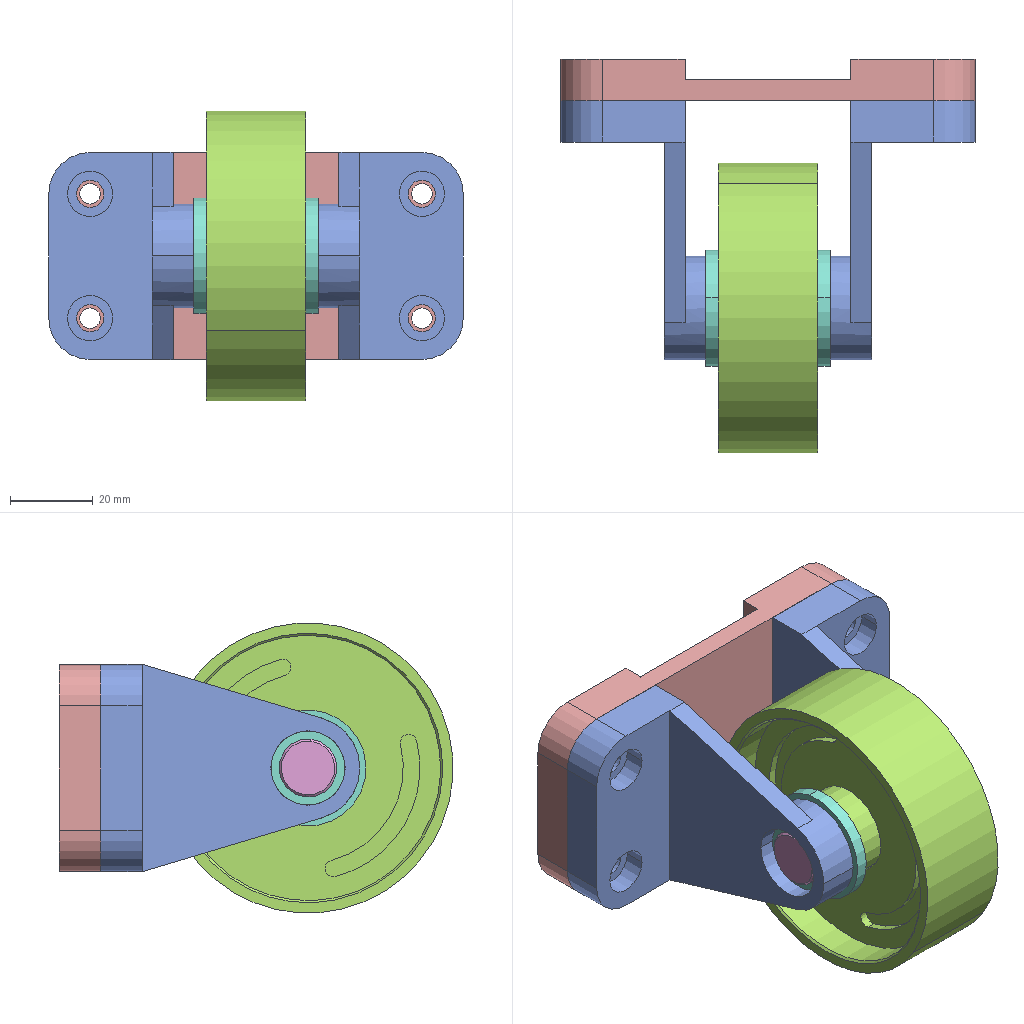Assembly | SolidWorks | 5 different items | 7 placed | box 100 x 95 x 70 mm
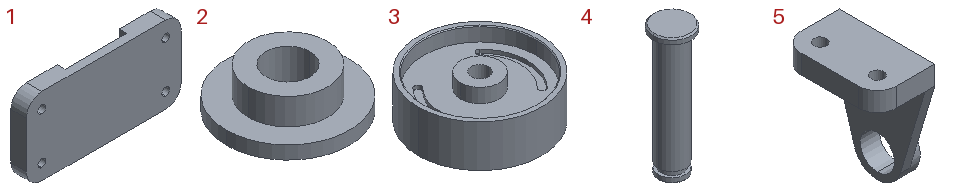Parts list (item | quantity | size | volume | features):
1 | x1 | 100 x 10 x 50 mm | 38356 mm3 | features 3DProfileFeature 1, Extrusion 1, Fillet 1, HoleWzd 1, ICE 1
2 | x2 | 28 x 28 x 9 mm | 2667 mm3 | features ICE 2, Extrusion 1
3 | x1 | 70 x 70 x 24 mm | 43680 mm3 | features ICE 3, MirrorPattern 2, Chamfer 1, Extrusion 1
4 | x1 | 14 x 14 x 48 mm | 3855 mm3 | features Chamfer 1, CutThin 1, Extrusion 1, ICE 1
5 | x2 | 35 x 50 x 62.5 mm | 22031 mm3 | features ICE 3, 3DProfileFeature 1, Extrusion 1, Fillet 1, HoleWzd 1
Mates (type | each side: item.copy, entity, surface, feature):
Concentric | 1.1 face cylinder M6 Tapped Hole1 | 5.1 face cylinder Cut-Extrude1 | 2 times
Coincident | 1.1 face plane Boss-Extrude1 | 5.1 face plane Boss-Extrude1
Concentric | 3.1 face cylinder Cut-Extrude1 | 2.1 face cylinder Cut-Extrude1
Concentric | 5.1 face cylinder Boss-Extrude3 | 3.1 face cylinder Cut-Extrude1
Coincident | 3.1 face plane Boss-Extrude1 | 2.1 face plane Boss-Extrude1
Coincident | 5.2 face plane Boss-Extrude4 | 2.1 face plane Boss-Extrude1
Concentric | 4.1 face cylinder Boss-Extrude1 | 2.1 face cylinder Cut-Extrude1
Coincident | 4.1 face plane Boss-Extrude2 | 2.1 face plane Boss-Extrude2